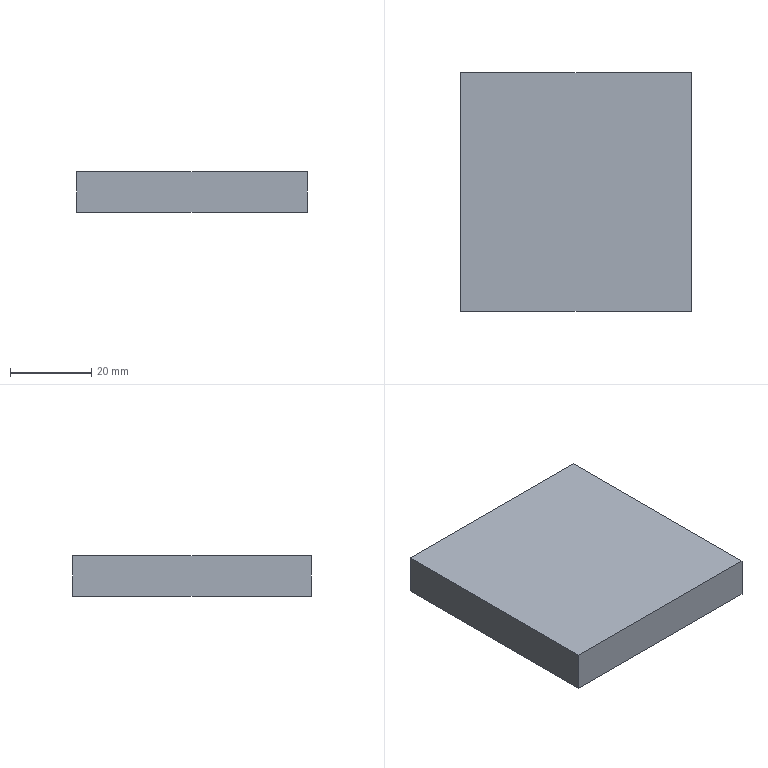Part | SolidWorks | features Extrusion 1 | 1 solid | 6 faces | box 56.969 x 58.85 x 10 mm | volume 33526 mm3 | plane 6
STEP:
#1=CARTESIAN_POINT('',(28.484,-29.425,0.));
#2=VERTEX_POINT('',#1);
#3=CARTESIAN_POINT('',(28.484,29.425,0.));
#4=VERTEX_POINT('',#3);
#5=CARTESIAN_POINT('',(28.484,29.425,0.));
#6=DIRECTION('',(0.,1.,0.));
#7=VECTOR('',#6,1000.);
#8=LINE('',#5,#7);
#9=EDGE_CURVE('',#2,#4,#8,.T.);
#10=ORIENTED_EDGE('',*,*,#9,.F.);
#11=CARTESIAN_POINT('',(28.484,-29.425,-10.));
#12=VERTEX_POINT('',#11);
#13=CARTESIAN_POINT('',(28.484,-29.425,-10.));
#14=DIRECTION('',(0.,0.,1.));
#15=VECTOR('',#14,1000.);
#16=LINE('',#13,#15);
#17=EDGE_CURVE('',#12,#2,#16,.T.);
#18=ORIENTED_EDGE('',*,*,#17,.F.);
#19=CARTESIAN_POINT('',(28.484,29.425,-10.));
#20=VERTEX_POINT('',#19);
#21=CARTESIAN_POINT('',(28.484,29.425,-10.));
#22=DIRECTION('',(0.,1.,0.));
#23=VECTOR('',#22,1000.);
#24=LINE('',#21,#23);
#25=EDGE_CURVE('',#12,#20,#24,.T.);
#26=ORIENTED_EDGE('',*,*,#25,.T.);
#27=CARTESIAN_POINT('',(28.484,29.425,-10.));
#28=DIRECTION('',(0.,0.,1.));
#29=VECTOR('',#28,1000.);
#30=LINE('',#27,#29);
#31=EDGE_CURVE('',#20,#4,#30,.T.);
#32=ORIENTED_EDGE('',*,*,#31,.T.);
#33=EDGE_LOOP('',(#10,#18,#26,#32));
#34=FACE_OUTER_BOUND('',#33,.T.);
#35=CARTESIAN_POINT('',(28.484,29.425,-10.));
#36=DIRECTION('',(1.,0.,0.));
#37=DIRECTION('',(0.,0.,-1.));
#38=AXIS2_PLACEMENT_3D('',#35,#36,#37);
#39=PLANE('',#38);
#40=ADVANCED_FACE('',(#34),#39,.T.);
#41=CARTESIAN_POINT('',(-28.484,-29.425,0.));
#42=VERTEX_POINT('',#41);
#43=CARTESIAN_POINT('',(-28.484,-29.425,0.));
#44=DIRECTION('',(1.,0.,0.));
#45=VECTOR('',#44,1000.);
#46=LINE('',#43,#45);
#47=EDGE_CURVE('',#42,#2,#46,.T.);
#48=ORIENTED_EDGE('',*,*,#47,.F.);
#49=CARTESIAN_POINT('',(-28.484,-29.425,-10.));
#50=VERTEX_POINT('',#49);
#51=CARTESIAN_POINT('',(-28.484,-29.425,-10.));
#52=DIRECTION('',(0.,0.,1.));
#53=VECTOR('',#52,1000.);
#54=LINE('',#51,#53);
#55=EDGE_CURVE('',#50,#42,#54,.T.);
#56=ORIENTED_EDGE('',*,*,#55,.F.);
#57=CARTESIAN_POINT('',(-28.484,-29.425,-10.));
#58=DIRECTION('',(1.,0.,0.));
#59=VECTOR('',#58,1000.);
#60=LINE('',#57,#59);
#61=EDGE_CURVE('',#50,#12,#60,.T.);
#62=ORIENTED_EDGE('',*,*,#61,.T.);
#63=ORIENTED_EDGE('',*,*,#17,.T.);
#64=EDGE_LOOP('',(#48,#56,#62,#63));
#65=FACE_OUTER_BOUND('',#64,.T.);
#66=CARTESIAN_POINT('',(-28.484,-29.425,-10.));
#67=DIRECTION('',(0.,-1.,0.));
#68=DIRECTION('',(0.,0.,-1.));
#69=AXIS2_PLACEMENT_3D('',#66,#67,#68);
#70=PLANE('',#69);
#71=ADVANCED_FACE('',(#65),#70,.T.);
#72=CARTESIAN_POINT('',(-28.484,29.425,0.));
#73=VERTEX_POINT('',#72);
#74=CARTESIAN_POINT('',(-28.484,29.425,0.));
#75=DIRECTION('',(0.,-1.,0.));
#76=VECTOR('',#75,1000.);
#77=LINE('',#74,#76);
#78=EDGE_CURVE('',#73,#42,#77,.T.);
#79=ORIENTED_EDGE('',*,*,#78,.F.);
#80=CARTESIAN_POINT('',(-28.484,29.425,-10.));
#81=VERTEX_POINT('',#80);
#82=CARTESIAN_POINT('',(-28.484,29.425,-10.));
#83=DIRECTION('',(0.,0.,1.));
#84=VECTOR('',#83,1000.);
#85=LINE('',#82,#84);
#86=EDGE_CURVE('',#81,#73,#85,.T.);
#87=ORIENTED_EDGE('',*,*,#86,.F.);
#88=CARTESIAN_POINT('',(-28.484,29.425,-10.));
#89=DIRECTION('',(0.,-1.,0.));
#90=VECTOR('',#89,1000.);
#91=LINE('',#88,#90);
#92=EDGE_CURVE('',#81,#50,#91,.T.);
#93=ORIENTED_EDGE('',*,*,#92,.T.);
#94=ORIENTED_EDGE('',*,*,#55,.T.);
#95=EDGE_LOOP('',(#79,#87,#93,#94));
#96=FACE_OUTER_BOUND('',#95,.T.);
#97=CARTESIAN_POINT('',(-28.484,29.425,-10.));
#98=DIRECTION('',(-1.,0.,0.));
#99=DIRECTION('',(0.,0.,1.));
#100=AXIS2_PLACEMENT_3D('',#97,#98,#99);
#101=PLANE('',#100);
#102=ADVANCED_FACE('',(#96),#101,.T.);
#103=CARTESIAN_POINT('',(-28.484,29.425,0.));
#104=DIRECTION('',(-1.,0.,0.));
#105=VECTOR('',#104,1000.);
#106=LINE('',#103,#105);
#107=EDGE_CURVE('',#4,#73,#106,.T.);
#108=ORIENTED_EDGE('',*,*,#107,.F.);
#109=ORIENTED_EDGE('',*,*,#31,.F.);
#110=CARTESIAN_POINT('',(-28.484,29.425,-10.));
#111=DIRECTION('',(-1.,0.,0.));
#112=VECTOR('',#111,1000.);
#113=LINE('',#110,#112);
#114=EDGE_CURVE('',#20,#81,#113,.T.);
#115=ORIENTED_EDGE('',*,*,#114,.T.);
#116=ORIENTED_EDGE('',*,*,#86,.T.);
#117=EDGE_LOOP('',(#108,#109,#115,#116));
#118=FACE_OUTER_BOUND('',#117,.T.);
#119=CARTESIAN_POINT('',(-28.484,29.425,-10.));
#120=DIRECTION('',(0.,1.,0.));
#121=DIRECTION('',(0.,0.,1.));
#122=AXIS2_PLACEMENT_3D('',#119,#120,#121);
#123=PLANE('',#122);
#124=ADVANCED_FACE('',(#118),#123,.T.);
#125=ORIENTED_EDGE('',*,*,#25,.F.);
#126=ORIENTED_EDGE('',*,*,#61,.F.);
#127=ORIENTED_EDGE('',*,*,#92,.F.);
#128=ORIENTED_EDGE('',*,*,#114,.F.);
#129=EDGE_LOOP('',(#125,#126,#127,#128));
#130=FACE_OUTER_BOUND('',#129,.T.);
#131=CARTESIAN_POINT('',(0.,0.,-10.));
#132=DIRECTION('',(0.,0.,1.));
#133=DIRECTION('',(1.,0.,0.));
#134=AXIS2_PLACEMENT_3D('',#131,#132,#133);
#135=PLANE('',#134);
#136=ADVANCED_FACE('',(#130),#135,.F.);
#137=ORIENTED_EDGE('',*,*,#9,.T.);
#138=ORIENTED_EDGE('',*,*,#107,.T.);
#139=ORIENTED_EDGE('',*,*,#78,.T.);
#140=ORIENTED_EDGE('',*,*,#47,.T.);
#141=EDGE_LOOP('',(#137,#138,#139,#140));
#142=FACE_OUTER_BOUND('',#141,.T.);
#143=CARTESIAN_POINT('',(0.,0.,0.));
#144=DIRECTION('',(0.,0.,1.));
#145=DIRECTION('',(1.,0.,0.));
#146=AXIS2_PLACEMENT_3D('',#143,#144,#145);
#147=PLANE('',#146);
#148=ADVANCED_FACE('',(#142),#147,.T.);
#149=CLOSED_SHELL('',(#40,#71,#102,#124,#136,#148));
#150=MANIFOLD_SOLID_BREP('',#149);
#151=CARTESIAN_POINT('',(0.,0.,0.));
#152=DIRECTION('',(0.,0.,1.));
#153=DIRECTION('',(1.,0.,0.));
#154=AXIS2_PLACEMENT_3D('',#151,#152,#153);
#155=(LENGTH_UNIT()NAMED_UNIT(*)SI_UNIT(.MILLI.,.METRE.));
#156=UNCERTAINTY_MEASURE_WITH_UNIT(LENGTH_MEASURE(0.00001),#155,'','');
#157=(NAMED_UNIT(*)PLANE_ANGLE_UNIT()SI_UNIT($,.RADIAN.));
#158=(NAMED_UNIT(*)SI_UNIT($,.STERADIAN.)SOLID_ANGLE_UNIT());
#159=(GEOMETRIC_REPRESENTATION_CONTEXT(3)GLOBAL_UNCERTAINTY_ASSIGNED_CONTEXT((#156))GLOBAL_UNIT_ASSIGNED_CONTEXT((#155,#157,#158))REPRESENTATION_CONTEXT('',''));
#160=ADVANCED_BREP_SHAPE_REPRESENTATION('',(#150,#154),#159);